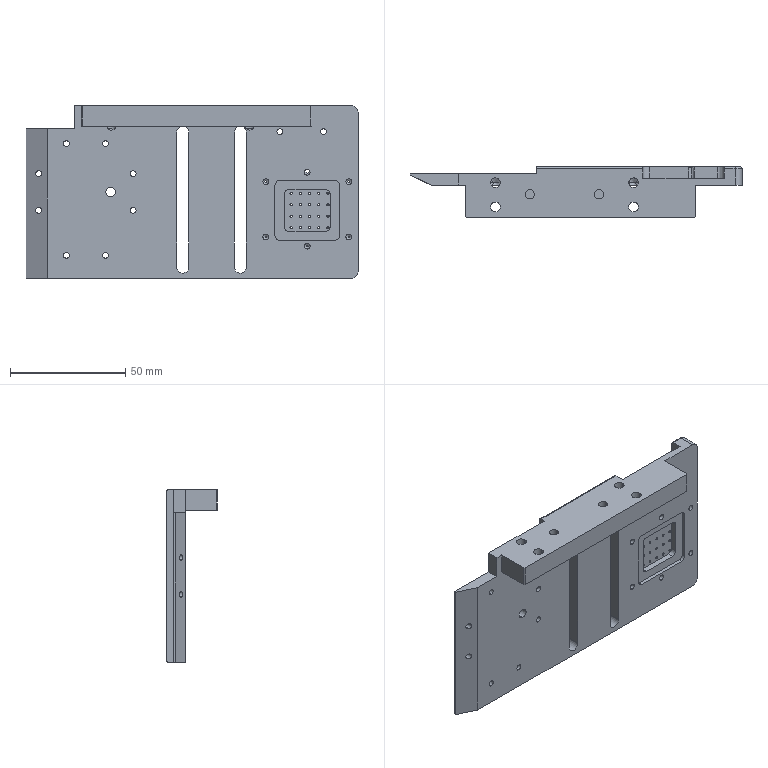Part | STEP file | 10000020488swp000-1 | 1 solid | 173 faces | box 144 x 22 x 75 mm | volume 68322 mm3 | cylinder 112 | plane 43 | cone 16 | torus 2 | commonest cylinder face diameters 1 x40 2.5 x32 4 x16 4.2 x10 5.2 x6 2 x4